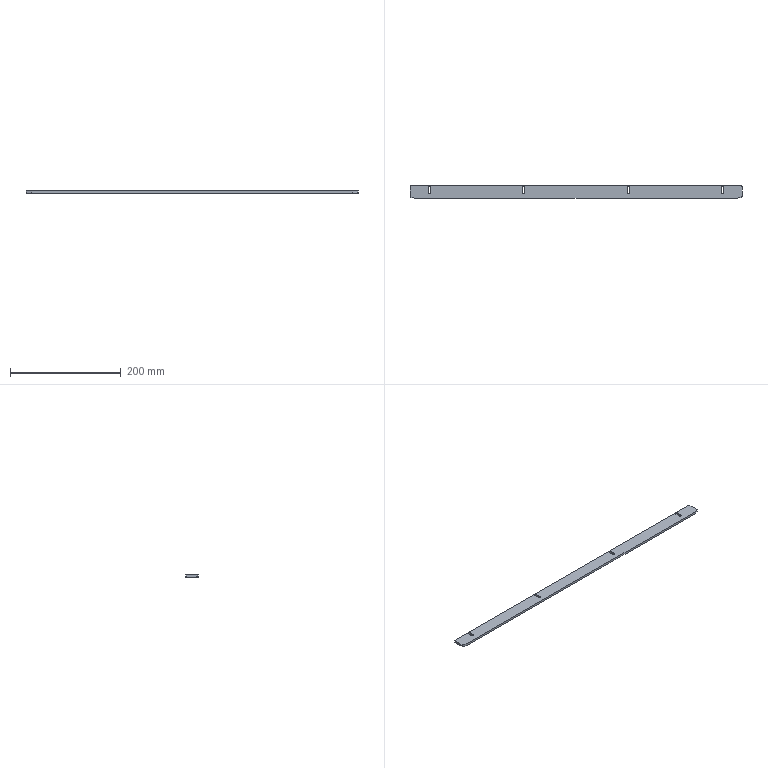Part | STEP file | 1 solid | 28 faces | box 600 x 23 x 4 mm | volume 54278 mm3 | plane 16 | cylinder 12 | commonest cylinder face diameters 4.5 x8 4 x4